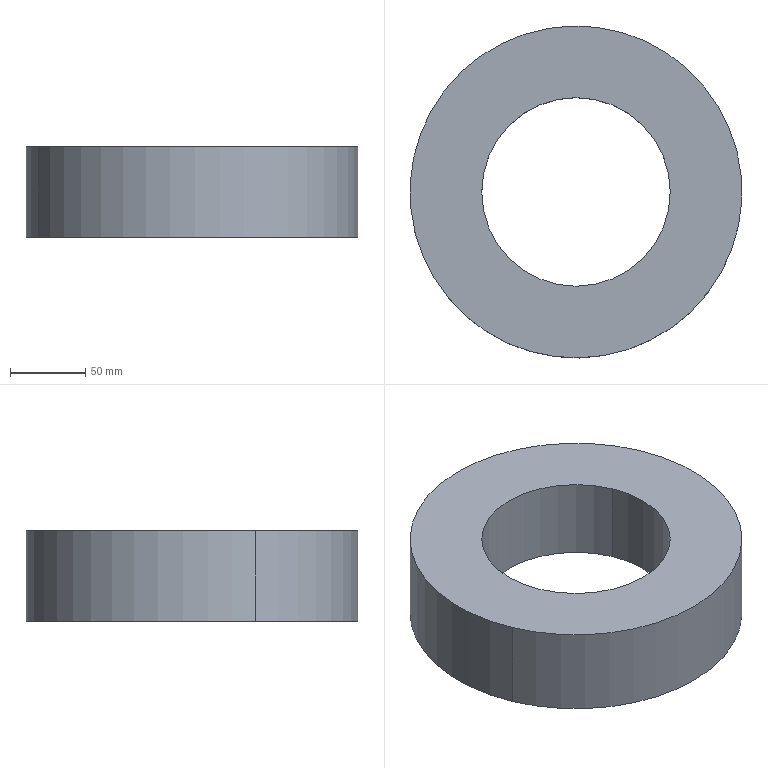Part | SolidWorks | features SplitBody 1 | 1 solid | 9 faces | box 220 x 220 x 60 mm | volume 1528876 mm3 | cylinder 6 | plane 3 | commonest cylinder face diameters 125 x2 140 x2 220 x2
STEP:
#1=CARTESIAN_POINT('',(3378.267,744.5,995.));
#2=VERTEX_POINT('',#1);
#3=CARTESIAN_POINT('',(3493.733,792.381,995.));
#4=VERTEX_POINT('',#3);
#5=CARTESIAN_POINT('',(3436.,768.44,995.));
#6=DIRECTION('',(0.,0.,1.));
#7=DIRECTION('',(0.9237,0.383,0.));
#8=AXIS2_PLACEMENT_3D('',#5,#6,#7);
#9=CIRCLE('',#8,62.5);
#10=EDGE_CURVE('',#2,#4,#9,.T.);
#11=ORIENTED_EDGE('',*,*,#10,.F.);
#12=CARTESIAN_POINT('',(3378.267,744.5,1050.));
#13=VERTEX_POINT('',#12);
#14=CARTESIAN_POINT('',(3378.267,744.5,990.));
#15=DIRECTION('',(0.,0.,1.));
#16=VECTOR('',#15,1000.);
#17=LINE('',#14,#16);
#18=EDGE_CURVE('',#2,#13,#17,.T.);
#19=ORIENTED_EDGE('',*,*,#18,.T.);
#20=CARTESIAN_POINT('',(3493.733,792.381,1050.));
#21=VERTEX_POINT('',#20);
#22=CARTESIAN_POINT('',(3436.,768.44,1050.));
#23=DIRECTION('',(0.,0.,1.));
#24=DIRECTION('',(0.9237,0.383,0.));
#25=AXIS2_PLACEMENT_3D('',#22,#23,#24);
#26=CIRCLE('',#25,62.5);
#27=EDGE_CURVE('',#13,#21,#26,.T.);
#28=ORIENTED_EDGE('',*,*,#27,.T.);
#29=CARTESIAN_POINT('',(3493.733,792.381,990.));
#30=DIRECTION('',(0.,0.,1.));
#31=VECTOR('',#30,1000.);
#32=LINE('',#29,#31);
#33=EDGE_CURVE('',#4,#21,#32,.T.);
#34=ORIENTED_EDGE('',*,*,#33,.F.);
#35=EDGE_LOOP('',(#11,#19,#28,#34));
#36=FACE_OUTER_BOUND('',#35,.T.);
#37=CARTESIAN_POINT('',(3436.,768.44,990.));
#38=DIRECTION('',(0.,0.,1.));
#39=DIRECTION('',(0.9237,0.383,0.));
#40=AXIS2_PLACEMENT_3D('',#37,#38,#39);
#41=CYLINDRICAL_SURFACE('',#40,62.5);
#42=ADVANCED_FACE('',(#36),#41,.F.);
#43=CARTESIAN_POINT('',(3537.61,810.576,990.));
#44=VERTEX_POINT('',#43);
#45=CARTESIAN_POINT('',(3334.39,726.305,990.));
#46=VERTEX_POINT('',#45);
#47=CARTESIAN_POINT('',(3436.,768.44,990.));
#48=DIRECTION('',(0.,0.,1.));
#49=DIRECTION('',(0.9237,0.383,0.));
#50=AXIS2_PLACEMENT_3D('',#47,#48,#49);
#51=CIRCLE('',#50,110.);
#52=EDGE_CURVE('',#44,#46,#51,.T.);
#53=ORIENTED_EDGE('',*,*,#52,.T.);
#54=CARTESIAN_POINT('',(3334.39,726.305,1050.));
#55=VERTEX_POINT('',#54);
#56=CARTESIAN_POINT('',(3334.39,726.305,990.));
#57=DIRECTION('',(0.,0.,1.));
#58=VECTOR('',#57,1000.);
#59=LINE('',#56,#58);
#60=EDGE_CURVE('',#46,#55,#59,.T.);
#61=ORIENTED_EDGE('',*,*,#60,.T.);
#62=CARTESIAN_POINT('',(3537.61,810.576,1050.));
#63=VERTEX_POINT('',#62);
#64=CARTESIAN_POINT('',(3436.,768.44,1050.));
#65=DIRECTION('',(0.,0.,-1.));
#66=DIRECTION('',(0.9237,0.383,0.));
#67=AXIS2_PLACEMENT_3D('',#64,#65,#66);
#68=CIRCLE('',#67,110.);
#69=EDGE_CURVE('',#55,#63,#68,.T.);
#70=ORIENTED_EDGE('',*,*,#69,.T.);
#71=CARTESIAN_POINT('',(3537.61,810.576,990.));
#72=DIRECTION('',(0.,0.,1.));
#73=VECTOR('',#72,1000.);
#74=LINE('',#71,#73);
#75=EDGE_CURVE('',#44,#63,#74,.T.);
#76=ORIENTED_EDGE('',*,*,#75,.F.);
#77=EDGE_LOOP('',(#53,#61,#70,#76));
#78=FACE_OUTER_BOUND('',#77,.T.);
#79=CARTESIAN_POINT('',(3436.,768.44,990.));
#80=DIRECTION('',(0.,0.,1.));
#81=DIRECTION('',(0.9237,0.383,0.));
#82=AXIS2_PLACEMENT_3D('',#79,#80,#81);
#83=CYLINDRICAL_SURFACE('',#82,110.);
#84=ADVANCED_FACE('',(#78),#83,.T.);
#85=CARTESIAN_POINT('',(3500.661,795.254,995.));
#86=VERTEX_POINT('',#85);
#87=CARTESIAN_POINT('',(3371.339,741.627,995.));
#88=VERTEX_POINT('',#87);
#89=CARTESIAN_POINT('',(3436.,768.44,995.));
#90=DIRECTION('',(0.,0.,-1.));
#91=DIRECTION('',(-0.9237,-0.383,0.));
#92=AXIS2_PLACEMENT_3D('',#89,#90,#91);
#93=CIRCLE('',#92,70.);
#94=EDGE_CURVE('',#86,#88,#93,.T.);
#95=ORIENTED_EDGE('',*,*,#94,.F.);
#96=CARTESIAN_POINT('',(3500.661,795.254,990.));
#97=VERTEX_POINT('',#96);
#98=CARTESIAN_POINT('',(3500.661,795.254,995.));
#99=DIRECTION('',(0.,0.,-1.));
#100=VECTOR('',#99,1000.);
#101=LINE('',#98,#100);
#102=EDGE_CURVE('',#86,#97,#101,.T.);
#103=ORIENTED_EDGE('',*,*,#102,.T.);
#104=CARTESIAN_POINT('',(3371.339,741.627,990.));
#105=VERTEX_POINT('',#104);
#106=CARTESIAN_POINT('',(3436.,768.44,990.));
#107=DIRECTION('',(0.,0.,1.));
#108=DIRECTION('',(-0.9237,-0.383,0.));
#109=AXIS2_PLACEMENT_3D('',#106,#107,#108);
#110=CIRCLE('',#109,70.);
#111=EDGE_CURVE('',#105,#97,#110,.T.);
#112=ORIENTED_EDGE('',*,*,#111,.F.);
#113=CARTESIAN_POINT('',(3371.339,741.627,995.));
#114=DIRECTION('',(0.,0.,-1.));
#115=VECTOR('',#114,1000.);
#116=LINE('',#113,#115);
#117=EDGE_CURVE('',#88,#105,#116,.T.);
#118=ORIENTED_EDGE('',*,*,#117,.F.);
#119=EDGE_LOOP('',(#95,#103,#112,#118));
#120=FACE_OUTER_BOUND('',#119,.T.);
#121=CARTESIAN_POINT('',(3436.,768.44,995.));
#122=DIRECTION('',(0.,0.,-1.));
#123=DIRECTION('',(-0.9237,-0.383,0.));
#124=AXIS2_PLACEMENT_3D('',#121,#122,#123);
#125=CYLINDRICAL_SURFACE('',#124,70.);
#126=ADVANCED_FACE('',(#120),#125,.F.);
#127=CARTESIAN_POINT('',(3436.,768.44,1050.));
#128=DIRECTION('',(0.,0.,1.));
#129=DIRECTION('',(0.9237,0.383,0.));
#130=AXIS2_PLACEMENT_3D('',#127,#128,#129);
#131=CIRCLE('',#130,62.5);
#132=EDGE_CURVE('',#21,#13,#131,.T.);
#133=ORIENTED_EDGE('',*,*,#132,.F.);
#134=ORIENTED_EDGE('',*,*,#27,.F.);
#135=EDGE_LOOP('',(#133,#134));
#136=FACE_BOUND('',#135,.T.);
#137=CARTESIAN_POINT('',(3436.,768.44,1050.));
#138=DIRECTION('',(0.,0.,-1.));
#139=DIRECTION('',(0.9237,0.383,0.));
#140=AXIS2_PLACEMENT_3D('',#137,#138,#139);
#141=CIRCLE('',#140,110.);
#142=EDGE_CURVE('',#63,#55,#141,.T.);
#143=ORIENTED_EDGE('',*,*,#142,.F.);
#144=ORIENTED_EDGE('',*,*,#69,.F.);
#145=EDGE_LOOP('',(#143,#144));
#146=FACE_OUTER_BOUND('',#145,.T.);
#147=CARTESIAN_POINT('',(3436.,768.44,1050.));
#148=DIRECTION('',(0.,0.,-1.));
#149=DIRECTION('',(-0.9237,-0.383,0.));
#150=AXIS2_PLACEMENT_3D('',#147,#148,#149);
#151=PLANE('',#150);
#152=ADVANCED_FACE('',(#136,#146),#151,.F.);
#153=ORIENTED_EDGE('',*,*,#18,.F.);
#154=CARTESIAN_POINT('',(3436.,768.44,995.));
#155=DIRECTION('',(0.,0.,1.));
#156=DIRECTION('',(0.9237,0.383,0.));
#157=AXIS2_PLACEMENT_3D('',#154,#155,#156);
#158=CIRCLE('',#157,62.5);
#159=EDGE_CURVE('',#4,#2,#158,.T.);
#160=ORIENTED_EDGE('',*,*,#159,.F.);
#161=ORIENTED_EDGE('',*,*,#33,.T.);
#162=ORIENTED_EDGE('',*,*,#132,.T.);
#163=EDGE_LOOP('',(#153,#160,#161,#162));
#164=FACE_OUTER_BOUND('',#163,.T.);
#165=CARTESIAN_POINT('',(3436.,768.44,990.));
#166=DIRECTION('',(0.,0.,1.));
#167=DIRECTION('',(0.9237,0.383,0.));
#168=AXIS2_PLACEMENT_3D('',#165,#166,#167);
#169=CYLINDRICAL_SURFACE('',#168,62.5);
#170=ADVANCED_FACE('',(#164),#169,.F.);
#171=ORIENTED_EDGE('',*,*,#60,.F.);
#172=CARTESIAN_POINT('',(3436.,768.44,990.));
#173=DIRECTION('',(0.,0.,1.));
#174=DIRECTION('',(0.9237,0.383,0.));
#175=AXIS2_PLACEMENT_3D('',#172,#173,#174);
#176=CIRCLE('',#175,110.);
#177=EDGE_CURVE('',#46,#44,#176,.T.);
#178=ORIENTED_EDGE('',*,*,#177,.T.);
#179=ORIENTED_EDGE('',*,*,#75,.T.);
#180=ORIENTED_EDGE('',*,*,#142,.T.);
#181=EDGE_LOOP('',(#171,#178,#179,#180));
#182=FACE_OUTER_BOUND('',#181,.T.);
#183=CARTESIAN_POINT('',(3436.,768.44,990.));
#184=DIRECTION('',(0.,0.,1.));
#185=DIRECTION('',(0.9237,0.383,0.));
#186=AXIS2_PLACEMENT_3D('',#183,#184,#185);
#187=CYLINDRICAL_SURFACE('',#186,110.);
#188=ADVANCED_FACE('',(#182),#187,.T.);
#189=CARTESIAN_POINT('',(3436.,768.44,995.));
#190=DIRECTION('',(0.,0.,-1.));
#191=DIRECTION('',(-0.9237,-0.383,0.));
#192=AXIS2_PLACEMENT_3D('',#189,#190,#191);
#193=CIRCLE('',#192,70.);
#194=EDGE_CURVE('',#88,#86,#193,.T.);
#195=ORIENTED_EDGE('',*,*,#194,.T.);
#196=ORIENTED_EDGE('',*,*,#94,.T.);
#197=EDGE_LOOP('',(#195,#196));
#198=FACE_OUTER_BOUND('',#197,.T.);
#199=ORIENTED_EDGE('',*,*,#159,.T.);
#200=ORIENTED_EDGE('',*,*,#10,.T.);
#201=EDGE_LOOP('',(#199,#200));
#202=FACE_BOUND('',#201,.T.);
#203=CARTESIAN_POINT('',(3436.,768.44,995.));
#204=DIRECTION('',(0.,0.,-1.));
#205=DIRECTION('',(-0.9237,-0.383,0.));
#206=AXIS2_PLACEMENT_3D('',#203,#204,#205);
#207=PLANE('',#206);
#208=ADVANCED_FACE('',(#198,#202),#207,.T.);
#209=ORIENTED_EDGE('',*,*,#52,.F.);
#210=ORIENTED_EDGE('',*,*,#177,.F.);
#211=EDGE_LOOP('',(#209,#210));
#212=FACE_OUTER_BOUND('',#211,.T.);
#213=ORIENTED_EDGE('',*,*,#111,.T.);
#214=CARTESIAN_POINT('',(3436.,768.44,990.));
#215=DIRECTION('',(0.,0.,1.));
#216=DIRECTION('',(-0.9237,-0.383,0.));
#217=AXIS2_PLACEMENT_3D('',#214,#215,#216);
#218=CIRCLE('',#217,70.);
#219=EDGE_CURVE('',#97,#105,#218,.T.);
#220=ORIENTED_EDGE('',*,*,#219,.T.);
#221=EDGE_LOOP('',(#213,#220));
#222=FACE_BOUND('',#221,.T.);
#223=CARTESIAN_POINT('',(3436.,768.44,990.));
#224=DIRECTION('',(0.,0.,-1.));
#225=DIRECTION('',(-0.9237,-0.383,0.));
#226=AXIS2_PLACEMENT_3D('',#223,#224,#225);
#227=PLANE('',#226);
#228=ADVANCED_FACE('',(#212,#222),#227,.T.);
#229=ORIENTED_EDGE('',*,*,#102,.F.);
#230=ORIENTED_EDGE('',*,*,#194,.F.);
#231=ORIENTED_EDGE('',*,*,#117,.T.);
#232=ORIENTED_EDGE('',*,*,#219,.F.);
#233=EDGE_LOOP('',(#229,#230,#231,#232));
#234=FACE_OUTER_BOUND('',#233,.T.);
#235=CARTESIAN_POINT('',(3436.,768.44,995.));
#236=DIRECTION('',(0.,0.,-1.));
#237=DIRECTION('',(-0.9237,-0.383,0.));
#238=AXIS2_PLACEMENT_3D('',#235,#236,#237);
#239=CYLINDRICAL_SURFACE('',#238,70.);
#240=ADVANCED_FACE('',(#234),#239,.F.);
#241=CLOSED_SHELL('',(#42,#84,#126,#152,#170,#188,#208,#228,#240));
#242=MANIFOLD_SOLID_BREP('',#241);
#243=CARTESIAN_POINT('',(0.,0.,0.));
#244=DIRECTION('',(0.,0.,1.));
#245=DIRECTION('',(1.,0.,0.));
#246=AXIS2_PLACEMENT_3D('',#243,#244,#245);
#247=(LENGTH_UNIT()NAMED_UNIT(*)SI_UNIT(.MILLI.,.METRE.));
#248=UNCERTAINTY_MEASURE_WITH_UNIT(LENGTH_MEASURE(0.00001),#247,'','');
#249=(NAMED_UNIT(*)PLANE_ANGLE_UNIT()SI_UNIT($,.RADIAN.));
#250=(NAMED_UNIT(*)SI_UNIT($,.STERADIAN.)SOLID_ANGLE_UNIT());
#251=(GEOMETRIC_REPRESENTATION_CONTEXT(3)GLOBAL_UNCERTAINTY_ASSIGNED_CONTEXT((#248))GLOBAL_UNIT_ASSIGNED_CONTEXT((#247,#249,#250))REPRESENTATION_CONTEXT('',''));
#252=ADVANCED_BREP_SHAPE_REPRESENTATION('',(#242,#246),#251);